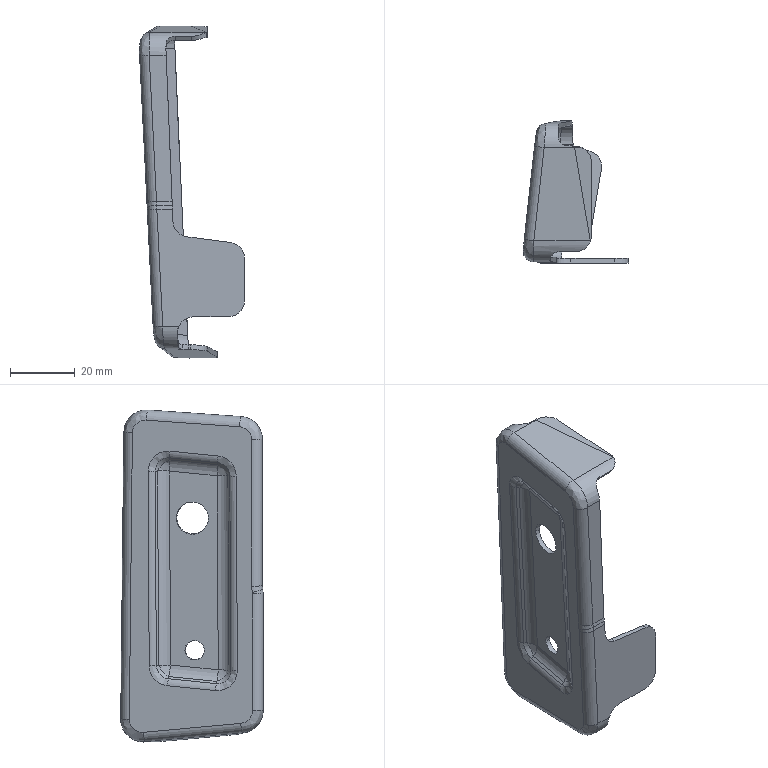Part | 1 solid | 143 faces | box 32.596 x 44.155 x 102.831 mm | volume 10241 mm3 | spline 88 | cylinder 44 | plane 11 | commonest cylinder face diameters 10 x10 3 x9 6 x9 13 x5 11 x4 14 x4